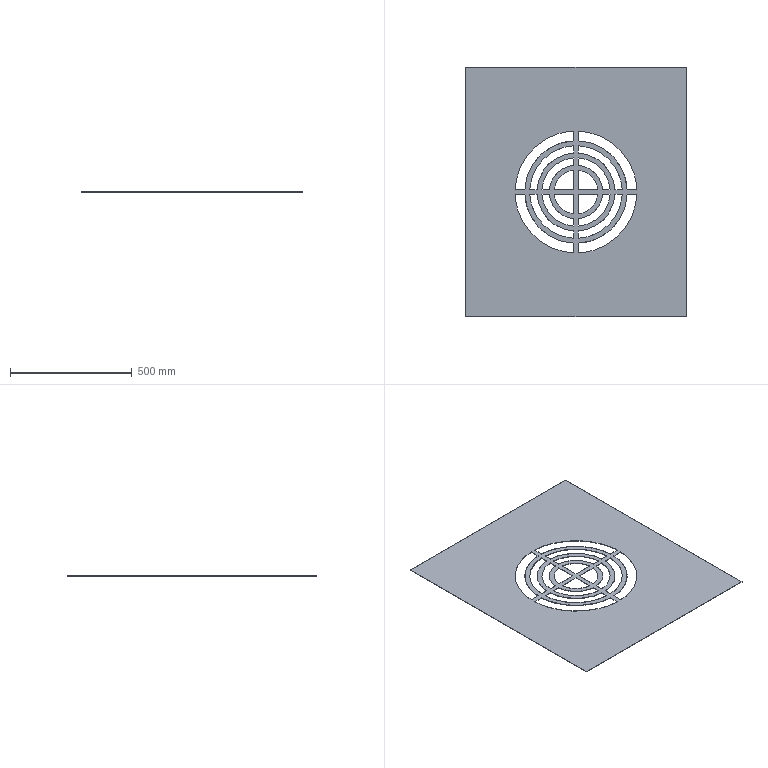Part | SolidWorks | features FlatPattern 1, MacroFeature 1, SMBaseFlange 1, SheetMetal 1 | 1 solid | 66 faces | box 904 x 1022 x 1.5 mm | volume 1198858 mm3 | plane 38 | spline 28